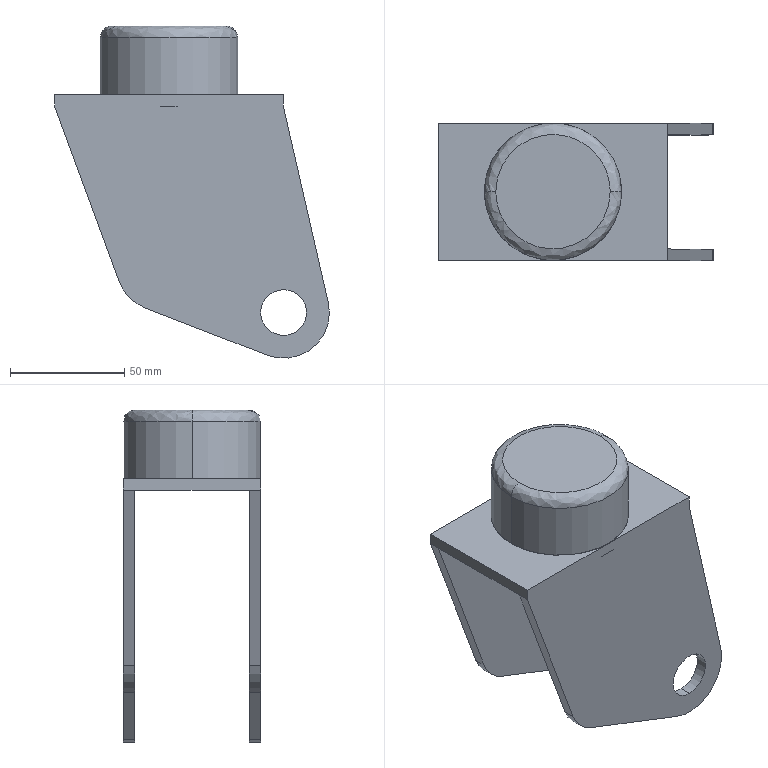Part | STEP file | 1 solid | 34 faces | box 120.126 x 60 x 145.273 mm | volume 22145 mm3 | plane 20 | cylinder 12 | spline 2 | commonest cylinder face diameters 20 x4 40 x4 60 x4